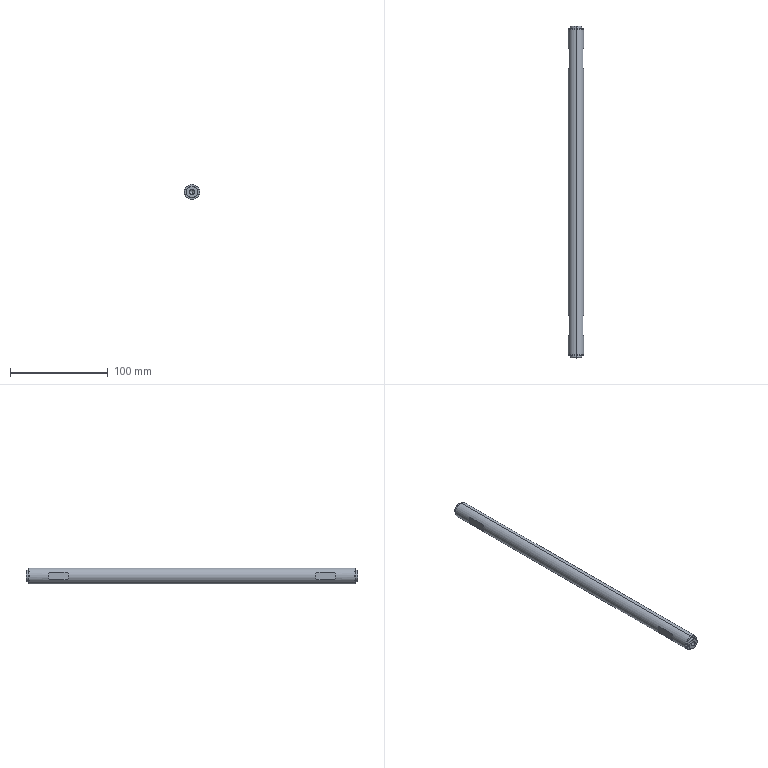Part | SolidWorks | features Chamfer 3, ICE 3, HoleWzd 2, Extrusion 1, MirrorPattern 1 | 1 solid | 38 faces | box 16 x 339 x 16 mm | volume 66505 mm3 | plane 16 | cone 12 | cylinder 10 | commonest cylinder face diameters 5 x4 12 x4 16 x2
STEP:
#1=CARTESIAN_POINT('',(0.,152.5,-2.5));
#2=VERTEX_POINT('',#1);
#3=CARTESIAN_POINT('',(0.,152.5,2.5));
#4=VERTEX_POINT('',#3);
#5=CARTESIAN_POINT('',(0.,152.5,0.));
#6=DIRECTION('',(0.,1.,0.));
#7=DIRECTION('',(0.,0.,1.));
#8=AXIS2_PLACEMENT_3D('',#5,#6,#7);
#9=CIRCLE('',#8,2.5);
#10=EDGE_CURVE('',#2,#4,#9,.T.);
#11=ORIENTED_EDGE('',*,*,#10,.F.);
#12=CARTESIAN_POINT('',(0.,169.5,-2.5));
#13=VERTEX_POINT('',#12);
#14=CARTESIAN_POINT('',(0.,169.5,-2.5));
#15=DIRECTION('',(0.,1.,0.));
#16=VECTOR('',#15,1000.);
#17=LINE('',#14,#16);
#18=EDGE_CURVE('',#2,#13,#17,.T.);
#19=ORIENTED_EDGE('',*,*,#18,.T.);
#20=CARTESIAN_POINT('',(0.,169.5,2.5));
#21=VERTEX_POINT('',#20);
#22=CARTESIAN_POINT('',(0.,169.5,0.));
#23=DIRECTION('',(0.,1.,0.));
#24=DIRECTION('',(0.,0.,1.));
#25=AXIS2_PLACEMENT_3D('',#22,#23,#24);
#26=CIRCLE('',#25,2.5);
#27=EDGE_CURVE('',#13,#21,#26,.T.);
#28=ORIENTED_EDGE('',*,*,#27,.T.);
#29=CARTESIAN_POINT('',(0.,169.5,2.5));
#30=DIRECTION('',(0.,1.,0.));
#31=VECTOR('',#30,1000.);
#32=LINE('',#29,#31);
#33=EDGE_CURVE('',#4,#21,#32,.T.);
#34=ORIENTED_EDGE('',*,*,#33,.F.);
#35=EDGE_LOOP('',(#11,#19,#28,#34));
#36=FACE_OUTER_BOUND('',#35,.T.);
#37=CARTESIAN_POINT('',(0.,169.5,0.));
#38=DIRECTION('',(0.,1.,0.));
#39=DIRECTION('',(0.,0.,1.));
#40=AXIS2_PLACEMENT_3D('',#37,#38,#39);
#41=CYLINDRICAL_SURFACE('',#40,2.5);
#42=ADVANCED_FACE('',(#36),#41,.F.);
#43=CARTESIAN_POINT('',(0.,150.998,0.));
#44=VERTEX_POINT('',#43);
#45=CARTESIAN_POINT('',(0.,152.5,2.5));
#46=DIRECTION('',(0.,0.515,0.8572));
#47=VECTOR('',#46,1000.);
#48=LINE('',#45,#47);
#49=EDGE_CURVE('',#44,#4,#48,.T.);
#50=ORIENTED_EDGE('',*,*,#49,.F.);
#51=CARTESIAN_POINT('',(0.,152.5,-2.5));
#52=DIRECTION('',(0.,0.515,-0.8572));
#53=VECTOR('',#52,1000.);
#54=LINE('',#51,#53);
#55=EDGE_CURVE('',#44,#2,#54,.T.);
#56=ORIENTED_EDGE('',*,*,#55,.T.);
#57=ORIENTED_EDGE('',*,*,#10,.T.);
#58=EDGE_LOOP('',(#50,#56,#57));
#59=FACE_OUTER_BOUND('',#58,.T.);
#60=CARTESIAN_POINT('',(0.,152.5,0.));
#61=DIRECTION('',(0.,1.,0.));
#62=DIRECTION('',(0.,0.,1.));
#63=AXIS2_PLACEMENT_3D('',#60,#61,#62);
#64=CONICAL_SURFACE('',#63,2.5,1.03);
#65=ADVANCED_FACE('',(#59),#64,.F.);
#66=CARTESIAN_POINT('',(0.,169.5,5.5));
#67=VERTEX_POINT('',#66);
#68=CARTESIAN_POINT('',(0.,169.5,-5.5));
#69=VERTEX_POINT('',#68);
#70=CARTESIAN_POINT('',(0.,169.5,0.));
#71=DIRECTION('',(0.,1.,0.));
#72=DIRECTION('',(0.,0.,1.));
#73=AXIS2_PLACEMENT_3D('',#70,#71,#72);
#74=CIRCLE('',#73,5.5);
#75=EDGE_CURVE('',#67,#69,#74,.T.);
#76=ORIENTED_EDGE('',*,*,#75,.F.);
#77=CARTESIAN_POINT('',(0.,169.,6.));
#78=VERTEX_POINT('',#77);
#79=CARTESIAN_POINT('',(0.,169.5,5.5));
#80=DIRECTION('',(0.,-0.7071,0.7071));
#81=VECTOR('',#80,1000.);
#82=LINE('',#79,#81);
#83=EDGE_CURVE('',#67,#78,#82,.T.);
#84=ORIENTED_EDGE('',*,*,#83,.T.);
#85=CARTESIAN_POINT('',(0.,169.,-6.));
#86=VERTEX_POINT('',#85);
#87=CARTESIAN_POINT('',(0.,169.,0.));
#88=DIRECTION('',(0.,-1.,0.));
#89=DIRECTION('',(0.,0.,1.));
#90=AXIS2_PLACEMENT_3D('',#87,#88,#89);
#91=CIRCLE('',#90,6.);
#92=EDGE_CURVE('',#86,#78,#91,.T.);
#93=ORIENTED_EDGE('',*,*,#92,.F.);
#94=CARTESIAN_POINT('',(0.,169.5,-5.5));
#95=DIRECTION('',(0.,-0.7071,-0.7071));
#96=VECTOR('',#95,1000.);
#97=LINE('',#94,#96);
#98=EDGE_CURVE('',#69,#86,#97,.T.);
#99=ORIENTED_EDGE('',*,*,#98,.F.);
#100=EDGE_LOOP('',(#76,#84,#93,#99));
#101=FACE_OUTER_BOUND('',#100,.T.);
#102=CARTESIAN_POINT('',(0.,169.5,0.));
#103=DIRECTION('',(0.,-1.,0.));
#104=DIRECTION('',(0.,0.,-1.));
#105=AXIS2_PLACEMENT_3D('',#102,#103,#104);
#106=CONICAL_SURFACE('',#105,5.5,0.7854);
#107=ADVANCED_FACE('',(#101),#106,.T.);
#108=ORIENTED_EDGE('',*,*,#92,.T.);
#109=CARTESIAN_POINT('',(0.,166.5,6.));
#110=VERTEX_POINT('',#109);
#111=CARTESIAN_POINT('',(0.,169.5,6.));
#112=DIRECTION('',(0.,-1.,0.));
#113=VECTOR('',#112,1000.);
#114=LINE('',#111,#113);
#115=EDGE_CURVE('',#78,#110,#114,.T.);
#116=ORIENTED_EDGE('',*,*,#115,.T.);
#117=CARTESIAN_POINT('',(0.,166.5,-6.));
#118=VERTEX_POINT('',#117);
#119=CARTESIAN_POINT('',(0.,166.5,0.));
#120=DIRECTION('',(0.,1.,0.));
#121=DIRECTION('',(0.,0.,1.));
#122=AXIS2_PLACEMENT_3D('',#119,#120,#121);
#123=CIRCLE('',#122,6.);
#124=EDGE_CURVE('',#110,#118,#123,.T.);
#125=ORIENTED_EDGE('',*,*,#124,.T.);
#126=CARTESIAN_POINT('',(0.,169.5,-6.));
#127=DIRECTION('',(0.,-1.,0.));
#128=VECTOR('',#127,1000.);
#129=LINE('',#126,#128);
#130=EDGE_CURVE('',#86,#118,#129,.T.);
#131=ORIENTED_EDGE('',*,*,#130,.F.);
#132=EDGE_LOOP('',(#108,#116,#125,#131));
#133=FACE_OUTER_BOUND('',#132,.T.);
#134=CARTESIAN_POINT('',(0.,169.5,0.));
#135=DIRECTION('',(0.,-1.,0.));
#136=DIRECTION('',(0.,0.,-1.));
#137=AXIS2_PLACEMENT_3D('',#134,#135,#136);
#138=CYLINDRICAL_SURFACE('',#137,6.);
#139=ADVANCED_FACE('',(#133),#138,.T.);
#140=CARTESIAN_POINT('',(0.,166.5,7.5));
#141=VERTEX_POINT('',#140);
#142=CARTESIAN_POINT('',(0.,166.5,-7.5));
#143=VERTEX_POINT('',#142);
#144=CARTESIAN_POINT('',(0.,166.5,0.));
#145=DIRECTION('',(0.,1.,0.));
#146=DIRECTION('',(0.,0.,1.));
#147=AXIS2_PLACEMENT_3D('',#144,#145,#146);
#148=CIRCLE('',#147,7.5);
#149=EDGE_CURVE('',#141,#143,#148,.T.);
#150=ORIENTED_EDGE('',*,*,#149,.F.);
#151=CARTESIAN_POINT('',(0.,166.,8.));
#152=VERTEX_POINT('',#151);
#153=CARTESIAN_POINT('',(0.,166.5,7.5));
#154=DIRECTION('',(0.,-0.7071,0.7071));
#155=VECTOR('',#154,1000.);
#156=LINE('',#153,#155);
#157=EDGE_CURVE('',#141,#152,#156,.T.);
#158=ORIENTED_EDGE('',*,*,#157,.T.);
#159=CARTESIAN_POINT('',(0.,166.,-8.));
#160=VERTEX_POINT('',#159);
#161=CARTESIAN_POINT('',(0.,166.,0.));
#162=DIRECTION('',(0.,-1.,0.));
#163=DIRECTION('',(0.,0.,1.));
#164=AXIS2_PLACEMENT_3D('',#161,#162,#163);
#165=CIRCLE('',#164,8.);
#166=EDGE_CURVE('',#160,#152,#165,.T.);
#167=ORIENTED_EDGE('',*,*,#166,.F.);
#168=CARTESIAN_POINT('',(0.,166.5,-7.5));
#169=DIRECTION('',(0.,-0.7071,-0.7071));
#170=VECTOR('',#169,1000.);
#171=LINE('',#168,#170);
#172=EDGE_CURVE('',#143,#160,#171,.T.);
#173=ORIENTED_EDGE('',*,*,#172,.F.);
#174=EDGE_LOOP('',(#150,#158,#167,#173));
#175=FACE_OUTER_BOUND('',#174,.T.);
#176=CARTESIAN_POINT('',(0.,166.5,0.));
#177=DIRECTION('',(0.,-1.,0.));
#178=DIRECTION('',(0.,0.,-1.));
#179=AXIS2_PLACEMENT_3D('',#176,#177,#178);
#180=CONICAL_SURFACE('',#179,7.5,0.7854);
#181=ADVANCED_FACE('',(#175),#180,.T.);
#182=CARTESIAN_POINT('',(0.,-152.5,2.5));
#183=VERTEX_POINT('',#182);
#184=CARTESIAN_POINT('',(0.,-152.5,-2.5));
#185=VERTEX_POINT('',#184);
#186=CARTESIAN_POINT('',(0.,-152.5,0.));
#187=DIRECTION('',(0.,-1.,0.));
#188=DIRECTION('',(0.,0.,-1.));
#189=AXIS2_PLACEMENT_3D('',#186,#187,#188);
#190=CIRCLE('',#189,2.5);
#191=EDGE_CURVE('',#183,#185,#190,.T.);
#192=ORIENTED_EDGE('',*,*,#191,.F.);
#193=CARTESIAN_POINT('',(0.,-169.5,2.5));
#194=VERTEX_POINT('',#193);
#195=CARTESIAN_POINT('',(0.,-169.5,2.5));
#196=DIRECTION('',(0.,-1.,0.));
#197=VECTOR('',#196,1000.);
#198=LINE('',#195,#197);
#199=EDGE_CURVE('',#183,#194,#198,.T.);
#200=ORIENTED_EDGE('',*,*,#199,.T.);
#201=CARTESIAN_POINT('',(0.,-169.5,-2.5));
#202=VERTEX_POINT('',#201);
#203=CARTESIAN_POINT('',(0.,-169.5,0.));
#204=DIRECTION('',(0.,-1.,0.));
#205=DIRECTION('',(0.,0.,-1.));
#206=AXIS2_PLACEMENT_3D('',#203,#204,#205);
#207=CIRCLE('',#206,2.5);
#208=EDGE_CURVE('',#194,#202,#207,.T.);
#209=ORIENTED_EDGE('',*,*,#208,.T.);
#210=CARTESIAN_POINT('',(0.,-169.5,-2.5));
#211=DIRECTION('',(0.,-1.,0.));
#212=VECTOR('',#211,1000.);
#213=LINE('',#210,#212);
#214=EDGE_CURVE('',#185,#202,#213,.T.);
#215=ORIENTED_EDGE('',*,*,#214,.F.);
#216=EDGE_LOOP('',(#192,#200,#209,#215));
#217=FACE_OUTER_BOUND('',#216,.T.);
#218=CARTESIAN_POINT('',(0.,-169.5,0.));
#219=DIRECTION('',(0.,-1.,0.));
#220=DIRECTION('',(0.,0.,-1.));
#221=AXIS2_PLACEMENT_3D('',#218,#219,#220);
#222=CYLINDRICAL_SURFACE('',#221,2.5);
#223=ADVANCED_FACE('',(#217),#222,.F.);
#224=CARTESIAN_POINT('',(0.,-150.998,0.));
#225=VERTEX_POINT('',#224);
#226=CARTESIAN_POINT('',(0.,-152.5,-2.5));
#227=DIRECTION('',(0.,-0.515,-0.8572));
#228=VECTOR('',#227,1000.);
#229=LINE('',#226,#228);
#230=EDGE_CURVE('',#225,#185,#229,.T.);
#231=ORIENTED_EDGE('',*,*,#230,.F.);
#232=CARTESIAN_POINT('',(0.,-152.5,2.5));
#233=DIRECTION('',(0.,-0.515,0.8572));
#234=VECTOR('',#233,1000.);
#235=LINE('',#232,#234);
#236=EDGE_CURVE('',#225,#183,#235,.T.);
#237=ORIENTED_EDGE('',*,*,#236,.T.);
#238=ORIENTED_EDGE('',*,*,#191,.T.);
#239=EDGE_LOOP('',(#231,#237,#238));
#240=FACE_OUTER_BOUND('',#239,.T.);
#241=CARTESIAN_POINT('',(0.,-152.5,0.));
#242=DIRECTION('',(0.,-1.,0.));
#243=DIRECTION('',(0.,0.,-1.));
#244=AXIS2_PLACEMENT_3D('',#241,#242,#243);
#245=CONICAL_SURFACE('',#244,2.5,1.03);
#246=ADVANCED_FACE('',(#240),#245,.F.);
#247=CARTESIAN_POINT('',(0.,-166.5,-7.5));
#248=VERTEX_POINT('',#247);
#249=CARTESIAN_POINT('',(0.,-166.5,7.5));
#250=VERTEX_POINT('',#249);
#251=CARTESIAN_POINT('',(0.,-166.5,0.));
#252=DIRECTION('',(0.,-1.,0.));
#253=DIRECTION('',(0.,0.,1.));
#254=AXIS2_PLACEMENT_3D('',#251,#252,#253);
#255=CIRCLE('',#254,7.5);
#256=EDGE_CURVE('',#248,#250,#255,.T.);
#257=ORIENTED_EDGE('',*,*,#256,.F.);
#258=CARTESIAN_POINT('',(0.,-166.,-8.));
#259=VERTEX_POINT('',#258);
#260=CARTESIAN_POINT('',(0.,-166.,-8.));
#261=DIRECTION('',(0.,0.7071,-0.7071));
#262=VECTOR('',#261,1000.);
#263=LINE('',#260,#262);
#264=EDGE_CURVE('',#248,#259,#263,.T.);
#265=ORIENTED_EDGE('',*,*,#264,.T.);
#266=CARTESIAN_POINT('',(0.,-166.,8.));
#267=VERTEX_POINT('',#266);
#268=CARTESIAN_POINT('',(0.,-166.,0.));
#269=DIRECTION('',(0.,1.,0.));
#270=DIRECTION('',(0.,0.,1.));
#271=AXIS2_PLACEMENT_3D('',#268,#269,#270);
#272=CIRCLE('',#271,8.);
#273=EDGE_CURVE('',#267,#259,#272,.T.);
#274=ORIENTED_EDGE('',*,*,#273,.F.);
#275=CARTESIAN_POINT('',(0.,-166.,8.));
#276=DIRECTION('',(0.,0.7071,0.7071));
#277=VECTOR('',#276,1000.);
#278=LINE('',#275,#277);
#279=EDGE_CURVE('',#250,#267,#278,.T.);
#280=ORIENTED_EDGE('',*,*,#279,.F.);
#281=EDGE_LOOP('',(#257,#265,#274,#280));
#282=FACE_OUTER_BOUND('',#281,.T.);
#283=CARTESIAN_POINT('',(0.,-166.,0.));
#284=DIRECTION('',(0.,1.,0.));
#285=DIRECTION('',(0.,0.,1.));
#286=AXIS2_PLACEMENT_3D('',#283,#284,#285);
#287=CONICAL_SURFACE('',#286,8.,0.7854);
#288=ADVANCED_FACE('',(#282),#287,.T.);
#289=CARTESIAN_POINT('',(0.,-169.5,-5.5));
#290=VERTEX_POINT('',#289);
#291=CARTESIAN_POINT('',(0.,-169.5,5.5));
#292=VERTEX_POINT('',#291);
#293=CARTESIAN_POINT('',(0.,-169.5,0.));
#294=DIRECTION('',(0.,-1.,0.));
#295=DIRECTION('',(0.,0.,-1.));
#296=AXIS2_PLACEMENT_3D('',#293,#294,#295);
#297=CIRCLE('',#296,5.5);
#298=EDGE_CURVE('',#290,#292,#297,.T.);
#299=ORIENTED_EDGE('',*,*,#298,.F.);
#300=CARTESIAN_POINT('',(0.,-169.,-6.));
#301=VERTEX_POINT('',#300);
#302=CARTESIAN_POINT('',(0.,-169.5,-5.5));
#303=DIRECTION('',(0.,0.7071,-0.7071));
#304=VECTOR('',#303,1000.);
#305=LINE('',#302,#304);
#306=EDGE_CURVE('',#290,#301,#305,.T.);
#307=ORIENTED_EDGE('',*,*,#306,.T.);
#308=CARTESIAN_POINT('',(0.,-169.,6.));
#309=VERTEX_POINT('',#308);
#310=CARTESIAN_POINT('',(0.,-169.,0.));
#311=DIRECTION('',(0.,1.,0.));
#312=DIRECTION('',(0.,0.,-1.));
#313=AXIS2_PLACEMENT_3D('',#310,#311,#312);
#314=CIRCLE('',#313,6.);
#315=EDGE_CURVE('',#309,#301,#314,.T.);
#316=ORIENTED_EDGE('',*,*,#315,.F.);
#317=CARTESIAN_POINT('',(0.,-169.5,5.5));
#318=DIRECTION('',(0.,0.7071,0.7071));
#319=VECTOR('',#318,1000.);
#320=LINE('',#317,#319);
#321=EDGE_CURVE('',#292,#309,#320,.T.);
#322=ORIENTED_EDGE('',*,*,#321,.F.);
#323=EDGE_LOOP('',(#299,#307,#316,#322));
#324=FACE_OUTER_BOUND('',#323,.T.);
#325=CARTESIAN_POINT('',(0.,-169.5,0.));
#326=DIRECTION('',(0.,1.,0.));
#327=DIRECTION('',(0.,0.,1.));
#328=AXIS2_PLACEMENT_3D('',#325,#326,#327);
#329=CONICAL_SURFACE('',#328,5.5,0.7854);
#330=ADVANCED_FACE('',(#324),#329,.T.);
#331=ORIENTED_EDGE('',*,*,#315,.T.);
#332=CARTESIAN_POINT('',(0.,-166.5,-6.));
#333=VERTEX_POINT('',#332);
#334=CARTESIAN_POINT('',(0.,-169.5,-6.));
#335=DIRECTION('',(0.,1.,0.));
#336=VECTOR('',#335,1000.);
#337=LINE('',#334,#336);
#338=EDGE_CURVE('',#301,#333,#337,.T.);
#339=ORIENTED_EDGE('',*,*,#338,.T.);
#340=CARTESIAN_POINT('',(0.,-166.5,6.));
#341=VERTEX_POINT('',#340);
#342=CARTESIAN_POINT('',(0.,-166.5,0.));
#343=DIRECTION('',(0.,-1.,0.));
#344=DIRECTION('',(0.,0.,1.));
#345=AXIS2_PLACEMENT_3D('',#342,#343,#344);
#346=CIRCLE('',#345,6.);
#347=EDGE_CURVE('',#333,#341,#346,.T.);
#348=ORIENTED_EDGE('',*,*,#347,.T.);
#349=CARTESIAN_POINT('',(0.,-169.5,6.));
#350=DIRECTION('',(0.,1.,0.));
#351=VECTOR('',#350,1000.);
#352=LINE('',#349,#351);
#353=EDGE_CURVE('',#309,#341,#352,.T.);
#354=ORIENTED_EDGE('',*,*,#353,.F.);
#355=EDGE_LOOP('',(#331,#339,#348,#354));
#356=FACE_OUTER_BOUND('',#355,.T.);
#357=CARTESIAN_POINT('',(0.,-169.5,0.));
#358=DIRECTION('',(0.,1.,0.));
#359=DIRECTION('',(0.,0.,1.));
#360=AXIS2_PLACEMENT_3D('',#357,#358,#359);
#361=CYLINDRICAL_SURFACE('',#360,6.);
#362=ADVANCED_FACE('',(#356),#361,.T.);
#363=CARTESIAN_POINT('',(7.,126.5,-3.873));
#364=VERTEX_POINT('',#363);
#365=CARTESIAN_POINT('',(7.,126.5,3.873));
#366=VERTEX_POINT('',#365);
#367=CARTESIAN_POINT('',(0.,126.5,0.));
#368=DIRECTION('',(0.,-1.,0.));
#369=DIRECTION('',(0.,0.,-1.));
#370=AXIS2_PLACEMENT_3D('',#367,#368,#369);
#371=CIRCLE('',#370,8.);
#372=EDGE_CURVE('',#364,#366,#371,.T.);
#373=ORIENTED_EDGE('',*,*,#372,.T.);
#374=CARTESIAN_POINT('',(7.,146.5,3.873));
#375=VERTEX_POINT('',#374);
#376=CARTESIAN_POINT('',(7.,126.5,3.873));
#377=DIRECTION('',(0.,1.,0.));
#378=VECTOR('',#377,1000.);
#379=LINE('',#376,#378);
#380=EDGE_CURVE('',#366,#375,#379,.T.);
#381=ORIENTED_EDGE('',*,*,#380,.T.);
#382=CARTESIAN_POINT('',(7.,146.5,-3.873));
#383=VERTEX_POINT('',#382);
#384=CARTESIAN_POINT('',(0.,146.5,0.));
#385=DIRECTION('',(0.,-1.,0.));
#386=DIRECTION('',(0.,0.,-1.));
#387=AXIS2_PLACEMENT_3D('',#384,#385,#386);
#388=CIRCLE('',#387,8.);
#389=EDGE_CURVE('',#383,#375,#388,.T.);
#390=ORIENTED_EDGE('',*,*,#389,.F.);
#391=CARTESIAN_POINT('',(7.,126.5,-3.873));
#392=DIRECTION('',(0.,1.,0.));
#393=VECTOR('',#392,1000.);
#394=LINE('',#391,#393);
#395=EDGE_CURVE('',#364,#383,#394,.T.);
#396=ORIENTED_EDGE('',*,*,#395,.F.);
#397=EDGE_LOOP('',(#373,#381,#390,#396));
#398=FACE_BOUND('',#397,.T.);
#399=CARTESIAN_POINT('',(7.,-126.5,-3.873));
#400=VERTEX_POINT('',#399);
#401=CARTESIAN_POINT('',(7.,-126.5,3.873));
#402=VERTEX_POINT('',#401);
#403=CARTESIAN_POINT('',(0.,-126.5,0.));
#404=DIRECTION('',(0.,-1.,0.));
#405=DIRECTION('',(0.,0.,-1.));
#406=AXIS2_PLACEMENT_3D('',#403,#404,#405);
#407=CIRCLE('',#406,8.);
#408=EDGE_CURVE('',#400,#402,#407,.T.);
#409=ORIENTED_EDGE('',*,*,#408,.F.);
#410=CARTESIAN_POINT('',(7.,-146.5,-3.873));
#411=VERTEX_POINT('',#410);
#412=CARTESIAN_POINT('',(7.,-126.5,-3.873));
#413=DIRECTION('',(0.,-1.,0.));
#414=VECTOR('',#413,1000.);
#415=LINE('',#412,#414);
#416=EDGE_CURVE('',#400,#411,#415,.T.);
#417=ORIENTED_EDGE('',*,*,#416,.T.);
#418=CARTESIAN_POINT('',(7.,-146.5,3.873));
#419=VERTEX_POINT('',#418);
#420=CARTESIAN_POINT('',(0.,-146.5,0.));
#421=DIRECTION('',(0.,-1.,0.));
#422=DIRECTION('',(0.,0.,-1.));
#423=AXIS2_PLACEMENT_3D('',#420,#421,#422);
#424=CIRCLE('',#423,8.);
#425=EDGE_CURVE('',#411,#419,#424,.T.);
#426=ORIENTED_EDGE('',*,*,#425,.T.);
#427=CARTESIAN_POINT('',(7.,-126.5,3.873));
#428=DIRECTION('',(0.,-1.,0.));
#429=VECTOR('',#428,1000.);
#430=LINE('',#427,#429);
#431=EDGE_CURVE('',#402,#419,#430,.T.);
#432=ORIENTED_EDGE('',*,*,#431,.F.);
#433=EDGE_LOOP('',(#409,#417,#426,#432));
#434=FACE_BOUND('',#433,.T.);
#435=ORIENTED_EDGE('',*,*,#166,.T.);
#436=CARTESIAN_POINT('',(0.,166.5,8.));
#437=DIRECTION('',(0.,-1.,0.));
#438=VECTOR('',#437,1000.);
#439=LINE('',#436,#438);
#440=EDGE_CURVE('',#152,#267,#439,.T.);
#441=ORIENTED_EDGE('',*,*,#440,.T.);
#442=ORIENTED_EDGE('',*,*,#273,.T.);
#443=CARTESIAN_POINT('',(0.,166.5,-8.));
#444=DIRECTION('',(0.,-1.,0.));
#445=VECTOR('',#444,1000.);
#446=LINE('',#443,#445);
#447=EDGE_CURVE('',#160,#259,#446,.T.);
#448=ORIENTED_EDGE('',*,*,#447,.F.);
#449=EDGE_LOOP('',(#435,#441,#442,#448));
#450=FACE_OUTER_BOUND('',#449,.T.);
#451=CARTESIAN_POINT('',(0.,166.5,0.));
#452=DIRECTION('',(0.,-1.,0.));
#453=DIRECTION('',(0.,0.,-1.));
#454=AXIS2_PLACEMENT_3D('',#451,#452,#453);
#455=CYLINDRICAL_SURFACE('',#454,8.);
#456=ADVANCED_FACE('',(#398,#434,#450),#455,.T.);
#457=ORIENTED_EDGE('',*,*,#440,.F.);
#458=CARTESIAN_POINT('',(0.,166.,0.));
#459=DIRECTION('',(0.,-1.,0.));
#460=DIRECTION('',(0.,0.,1.));
#461=AXIS2_PLACEMENT_3D('',#458,#459,#460);
#462=CIRCLE('',#461,8.);
#463=EDGE_CURVE('',#152,#160,#462,.T.);
#464=ORIENTED_EDGE('',*,*,#463,.T.);
#465=ORIENTED_EDGE('',*,*,#447,.T.);
#466=CARTESIAN_POINT('',(0.,-166.,0.));
#467=DIRECTION('',(0.,1.,0.));
#468=DIRECTION('',(0.,0.,1.));
#469=AXIS2_PLACEMENT_3D('',#466,#467,#468);
#470=CIRCLE('',#469,8.);
#471=EDGE_CURVE('',#259,#267,#470,.T.);
#472=ORIENTED_EDGE('',*,*,#471,.T.);
#473=EDGE_LOOP('',(#457,#464,#465,#472));
#474=FACE_OUTER_BOUND('',#473,.T.);
#475=CARTESIAN_POINT('',(-7.,126.5,3.873));
#476=VERTEX_POINT('',#475);
#477=CARTESIAN_POINT('',(-7.,126.5,-3.873));
#478=VERTEX_POINT('',#477);
#479=CARTESIAN_POINT('',(0.,126.5,0.));
#480=DIRECTION('',(0.,-1.,0.));
#481=DIRECTION('',(0.,0.,-1.));
#482=AXIS2_PLACEMENT_3D('',#479,#480,#481);
#483=CIRCLE('',#482,8.);
#484=EDGE_CURVE('',#476,#478,#483,.T.);
#485=ORIENTED_EDGE('',*,*,#484,.T.);
#486=CARTESIAN_POINT('',(-7.,146.5,-3.873));
#487=VERTEX_POINT('',#486);
#488=CARTESIAN_POINT('',(-7.,126.5,-3.873));
#489=DIRECTION('',(0.,1.,0.));
#490=VECTOR('',#489,1000.);
#491=LINE('',#488,#490);
#492=EDGE_CURVE('',#478,#487,#491,.T.);
#493=ORIENTED_EDGE('',*,*,#492,.T.);
#494=CARTESIAN_POINT('',(-7.,146.5,3.873));
#495=VERTEX_POINT('',#494);
#496=CARTESIAN_POINT('',(0.,146.5,0.));
#497=DIRECTION('',(0.,-1.,0.));
#498=DIRECTION('',(0.,0.,-1.));
#499=AXIS2_PLACEMENT_3D('',#496,#497,#498);
#500=CIRCLE('',#499,8.);
#501=EDGE_CURVE('',#495,#487,#500,.T.);
#502=ORIENTED_EDGE('',*,*,#501,.F.);
#503=CARTESIAN_POINT('',(-7.,126.5,3.873));
#504=DIRECTION('',(0.,1.,0.));
#505=VECTOR('',#504,1000.);
#506=LINE('',#503,#505);
#507=EDGE_CURVE('',#476,#495,#506,.T.);
#508=ORIENTED_EDGE('',*,*,#507,.F.);
#509=EDGE_LOOP('',(#485,#493,#502,#508));
#510=FACE_BOUND('',#509,.T.);
#511=CARTESIAN_POINT('',(-7.,-126.5,3.873));
#512=VERTEX_POINT('',#511);
#513=CARTESIAN_POINT('',(-7.,-126.5,-3.873));
#514=VERTEX_POINT('',#513);
#515=CARTESIAN_POINT('',(0.,-126.5,0.));
#516=DIRECTION('',(0.,-1.,0.));
#517=DIRECTION('',(0.,0.,-1.));
#518=AXIS2_PLACEMENT_3D('',#515,#516,#517);
#519=CIRCLE('',#518,8.);
#520=EDGE_CURVE('',#512,#514,#519,.T.);
#521=ORIENTED_EDGE('',*,*,#520,.F.);
#522=CARTESIAN_POINT('',(-7.,-146.5,3.873));
#523=VERTEX_POINT('',#522);
#524=CARTESIAN_POINT('',(-7.,-126.5,3.873));
#525=DIRECTION('',(0.,-1.,0.));
#526=VECTOR('',#525,1000.);
#527=LINE('',#524,#526);
#528=EDGE_CURVE('',#512,#523,#527,.T.);
#529=ORIENTED_EDGE('',*,*,#528,.T.);
#530=CARTESIAN_POINT('',(-7.,-146.5,-3.873));
#531=VERTEX_POINT('',#530);
#532=CARTESIAN_POINT('',(0.,-146.5,0.));
#533=DIRECTION('',(0.,-1.,0.));
#534=DIRECTION('',(0.,0.,-1.));
#535=AXIS2_PLACEMENT_3D('',#532,#533,#534);
#536=CIRCLE('',#535,8.);
#537=EDGE_CURVE('',#523,#531,#536,.T.);
#538=ORIENTED_EDGE('',*,*,#537,.T.);
#539=CARTESIAN_POINT('',(-7.,-126.5,-3.873));
#540=DIRECTION('',(0.,-1.,0.));
#541=VECTOR('',#540,1000.);
#542=LINE('',#539,#541);
#543=EDGE_CURVE('',#514,#531,#542,.T.);
#544=ORIENTED_EDGE('',*,*,#543,.F.);
#545=EDGE_LOOP('',(#521,#529,#538,#544));
#546=FACE_BOUND('',#545,.T.);
#547=CARTESIAN_POINT('',(0.,166.5,0.));
#548=DIRECTION('',(0.,-1.,0.));
#549=DIRECTION('',(0.,0.,-1.));
#550=AXIS2_PLACEMENT_3D('',#547,#548,#549);
#551=CYLINDRICAL_SURFACE('',#550,8.);
#552=ADVANCED_FACE('',(#474,#510,#546),#551,.T.);
#553=CARTESIAN_POINT('',(0.,166.5,0.));
#554=DIRECTION('',(0.,1.,0.));
#555=DIRECTION('',(0.,0.,1.));
#556=AXIS2_PLACEMENT_3D('',#553,#554,#555);
#557=CIRCLE('',#556,7.5);
#558=EDGE_CURVE('',#143,#141,#557,.T.);
#559=ORIENTED_EDGE('',*,*,#558,.T.);
#560=ORIENTED_EDGE('',*,*,#149,.T.);
#561=EDGE_LOOP('',(#559,#560));
#562=FACE_OUTER_BOUND('',#561,.T.);
#563=CARTESIAN_POINT('',(0.,166.5,0.));
#564=DIRECTION('',(0.,1.,0.));
#565=DIRECTION('',(0.,0.,1.));
#566=AXIS2_PLACEMENT_3D('',#563,#564,#565);
#567=CIRCLE('',#566,6.);
#568=EDGE_CURVE('',#118,#110,#567,.T.);
#569=ORIENTED_EDGE('',*,*,#568,.F.);
#570=ORIENTED_EDGE('',*,*,#124,.F.);
#571=EDGE_LOOP('',(#569,#570));
#572=FACE_BOUND('',#571,.T.);
#573=CARTESIAN_POINT('',(0.,166.5,0.));
#574=DIRECTION('',(0.,1.,0.));
#575=DIRECTION('',(0.,0.,1.));
#576=AXIS2_PLACEMENT_3D('',#573,#574,#575);
#577=PLANE('',#576);
#578=ADVANCED_FACE('',(#562,#572),#577,.T.);
#579=CARTESIAN_POINT('',(0.,-166.5,0.));
#580=DIRECTION('',(0.,-1.,0.));
#581=DIRECTION('',(0.,0.,1.));
#582=AXIS2_PLACEMENT_3D('',#579,#580,#581);
#583=CIRCLE('',#582,7.5);
#584=EDGE_CURVE('',#250,#248,#583,.T.);
#585=ORIENTED_EDGE('',*,*,#584,.T.);
#586=ORIENTED_EDGE('',*,*,#256,.T.);
#587=EDGE_LOOP('',(#585,#586));
#588=FACE_OUTER_BOUND('',#587,.T.);
#589=CARTESIAN_POINT('',(0.,-166.5,0.));
#590=DIRECTION('',(0.,-1.,0.));
#591=DIRECTION('',(0.,0.,1.));
#592=AXIS2_PLACEMENT_3D('',#589,#590,#591);
#593=CIRCLE('',#592,6.);
#594=EDGE_CURVE('',#341,#333,#593,.T.);
#595=ORIENTED_EDGE('',*,*,#594,.F.);
#596=ORIENTED_EDGE('',*,*,#347,.F.);
#597=EDGE_LOOP('',(#595,#596));
#598=FACE_BOUND('',#597,.T.);
#599=CARTESIAN_POINT('',(0.,-166.5,0.));
#600=DIRECTION('',(0.,1.,0.));
#601=DIRECTION('',(0.,0.,1.));
#602=AXIS2_PLACEMENT_3D('',#599,#600,#601);
#603=PLANE('',#602);
#604=ADVANCED_FACE('',(#588,#598),#603,.F.);
#605=ORIENTED_EDGE('',*,*,#338,.F.);
#606=CARTESIAN_POINT('',(0.,-169.,0.));
#607=DIRECTION('',(0.,1.,0.));
#608=DIRECTION('',(0.,0.,-1.));
#609=AXIS2_PLACEMENT_3D('',#606,#607,#608);
#610=CIRCLE('',#609,6.);
#611=EDGE_CURVE('',#301,#309,#610,.T.);
#612=ORIENTED_EDGE('',*,*,#611,.T.);
#613=ORIENTED_EDGE('',*,*,#353,.T.);
#614=ORIENTED_EDGE('',*,*,#594,.T.);
#615=EDGE_LOOP('',(#605,#612,#613,#614));
#616=FACE_OUTER_BOUND('',#615,.T.);
#617=CARTESIAN_POINT('',(0.,-169.5,0.));
#618=DIRECTION('',(0.,1.,0.));
#619=DIRECTION('',(0.,0.,1.));
#620=AXIS2_PLACEMENT_3D('',#617,#618,#619);
#621=CYLINDRICAL_SURFACE('',#620,6.);
#622=ADVANCED_FACE('',(#616),#621,.T.);
#623=CARTESIAN_POINT('',(0.,-169.5,0.));
#624=DIRECTION('',(0.,-1.,0.));
#625=DIRECTION('',(0.,0.,-1.));
#626=AXIS2_PLACEMENT_3D('',#623,#624,#625);
#627=CIRCLE('',#626,2.5);
#628=EDGE_CURVE('',#202,#194,#627,.T.);
#629=ORIENTED_EDGE('',*,*,#628,.F.);
#630=ORIENTED_EDGE('',*,*,#208,.F.);
#631=EDGE_LOOP('',(#629,#630));
#632=FACE_BOUND('',#631,.T.);
#633=CARTESIAN_POINT('',(0.,-169.5,0.));
#634=DIRECTION('',(0.,-1.,0.));
#635=DIRECTION('',(0.,0.,-1.));
#636=AXIS2_PLACEMENT_3D('',#633,#634,#635);
#637=CIRCLE('',#636,5.5);
#638=EDGE_CURVE('',#292,#290,#637,.T.);
#639=ORIENTED_EDGE('',*,*,#638,.T.);
#640=ORIENTED_EDGE('',*,*,#298,.T.);
#641=EDGE_LOOP('',(#639,#640));
#642=FACE_OUTER_BOUND('',#641,.T.);
#643=CARTESIAN_POINT('',(0.,-169.5,0.));
#644=DIRECTION('',(0.,-1.,0.));
#645=DIRECTION('',(0.,0.,-1.));
#646=AXIS2_PLACEMENT_3D('',#643,#644,#645);
#647=PLANE('',#646);
#648=ADVANCED_FACE('',(#632,#642),#647,.T.);
#649=ORIENTED_EDGE('',*,*,#306,.F.);
#650=ORIENTED_EDGE('',*,*,#638,.F.);
#651=ORIENTED_EDGE('',*,*,#321,.T.);
#652=ORIENTED_EDGE('',*,*,#611,.F.);
#653=EDGE_LOOP('',(#649,#650,#651,#652));
#654=FACE_OUTER_BOUND('',#653,.T.);
#655=CARTESIAN_POINT('',(0.,-169.5,0.));
#656=DIRECTION('',(0.,1.,0.));
#657=DIRECTION('',(0.,0.,1.));
#658=AXIS2_PLACEMENT_3D('',#655,#656,#657);
#659=CONICAL_SURFACE('',#658,5.5,0.7854);
#660=ADVANCED_FACE('',(#654),#659,.T.);
#661=ORIENTED_EDGE('',*,*,#264,.F.);
#662=ORIENTED_EDGE('',*,*,#584,.F.);
#663=ORIENTED_EDGE('',*,*,#279,.T.);
#664=ORIENTED_EDGE('',*,*,#471,.F.);
#665=EDGE_LOOP('',(#661,#662,#663,#664));
#666=FACE_OUTER_BOUND('',#665,.T.);
#667=CARTESIAN_POINT('',(0.,-166.,0.));
#668=DIRECTION('',(0.,1.,0.));
#669=DIRECTION('',(0.,0.,1.));
#670=AXIS2_PLACEMENT_3D('',#667,#668,#669);
#671=CONICAL_SURFACE('',#670,8.,0.7854);
#672=ADVANCED_FACE('',(#666),#671,.T.);
#673=CARTESIAN_POINT('',(-7.,-146.5,3.873));
#674=DIRECTION('',(0.,0.,1.));
#675=VECTOR('',#674,1000.);
#676=LINE('',#673,#675);
#677=EDGE_CURVE('',#531,#523,#676,.T.);
#678=ORIENTED_EDGE('',*,*,#677,.T.);
#679=ORIENTED_EDGE('',*,*,#528,.F.);
#680=CARTESIAN_POINT('',(-7.,-126.5,3.873));
#681=DIRECTION('',(0.,0.,1.));
#682=VECTOR('',#681,1000.);
#683=LINE('',#680,#682);
#684=EDGE_CURVE('',#514,#512,#683,.T.);
#685=ORIENTED_EDGE('',*,*,#684,.F.);
#686=ORIENTED_EDGE('',*,*,#543,.T.);
#687=EDGE_LOOP('',(#678,#679,#685,#686));
#688=FACE_OUTER_BOUND('',#687,.T.);
#689=CARTESIAN_POINT('',(-7.,-126.5,3.873));
#690=DIRECTION('',(1.,0.,0.));
#691=DIRECTION('',(0.,0.,-1.));
#692=AXIS2_PLACEMENT_3D('',#689,#690,#691);
#693=PLANE('',#692);
#694=ADVANCED_FACE('',(#688),#693,.F.);
#695=ORIENTED_EDGE('',*,*,#520,.T.);
#696=ORIENTED_EDGE('',*,*,#684,.T.);
#697=EDGE_LOOP('',(#695,#696));
#698=FACE_OUTER_BOUND('',#697,.T.);
#699=CARTESIAN_POINT('',(0.,-126.5,0.));
#700=DIRECTION('',(0.,-1.,0.));
#701=DIRECTION('',(0.,0.,-1.));
#702=AXIS2_PLACEMENT_3D('',#699,#700,#701);
#703=PLANE('',#702);
#704=ADVANCED_FACE('',(#698),#703,.T.);
#705=ORIENTED_EDGE('',*,*,#537,.F.);
#706=ORIENTED_EDGE('',*,*,#677,.F.);
#707=EDGE_LOOP('',(#705,#706));
#708=FACE_OUTER_BOUND('',#707,.T.);
#709=CARTESIAN_POINT('',(0.,-146.5,0.));
#710=DIRECTION('',(0.,-1.,0.));
#711=DIRECTION('',(0.,0.,-1.));
#712=AXIS2_PLACEMENT_3D('',#709,#710,#711);
#713=PLANE('',#712);
#714=ADVANCED_FACE('',(#708),#713,.F.);
#715=CARTESIAN_POINT('',(7.,-146.5,3.873));
#716=DIRECTION('',(0.,0.,-1.));
#717=VECTOR('',#716,1000.);
#718=LINE('',#715,#717);
#719=EDGE_CURVE('',#419,#411,#718,.T.);
#720=ORIENTED_EDGE('',*,*,#719,.T.);
#721=ORIENTED_EDGE('',*,*,#416,.F.);
#722=CARTESIAN_POINT('',(7.,-126.5,3.873));
#723=DIRECTION('',(0.,0.,-1.));
#724=VECTOR('',#723,1000.);
#725=LINE('',#722,#724);
#726=EDGE_CURVE('',#402,#400,#725,.T.);
#727=ORIENTED_EDGE('',*,*,#726,.F.);
#728=ORIENTED_EDGE('',*,*,#431,.T.);
#729=EDGE_LOOP('',(#720,#721,#727,#728));
#730=FACE_OUTER_BOUND('',#729,.T.);
#731=CARTESIAN_POINT('',(7.,-126.5,3.873));
#732=DIRECTION('',(-1.,0.,0.));
#733=DIRECTION('',(0.,0.,1.));
#734=AXIS2_PLACEMENT_3D('',#731,#732,#733);
#735=PLANE('',#734);
#736=ADVANCED_FACE('',(#730),#735,.F.);
#737=ORIENTED_EDGE('',*,*,#408,.T.);
#738=ORIENTED_EDGE('',*,*,#726,.T.);
#739=EDGE_LOOP('',(#737,#738));
#740=FACE_OUTER_BOUND('',#739,.T.);
#741=CARTESIAN_POINT('',(0.,-126.5,0.));
#742=DIRECTION('',(0.,-1.,0.));
#743=DIRECTION('',(0.,0.,-1.));
#744=AXIS2_PLACEMENT_3D('',#741,#742,#743);
#745=PLANE('',#744);
#746=ADVANCED_FACE('',(#740),#745,.T.);
#747=ORIENTED_EDGE('',*,*,#425,.F.);
#748=ORIENTED_EDGE('',*,*,#719,.F.);
#749=EDGE_LOOP('',(#747,#748));
#750=FACE_OUTER_BOUND('',#749,.T.);
#751=CARTESIAN_POINT('',(0.,-146.5,0.));
#752=DIRECTION('',(0.,-1.,0.));
#753=DIRECTION('',(0.,0.,-1.));
#754=AXIS2_PLACEMENT_3D('',#751,#752,#753);
#755=PLANE('',#754);
#756=ADVANCED_FACE('',(#750),#755,.F.);
#757=ORIENTED_EDGE('',*,*,#236,.F.);
#758=ORIENTED_EDGE('',*,*,#230,.T.);
#759=CARTESIAN_POINT('',(0.,-152.5,0.));
#760=DIRECTION('',(0.,-1.,0.));
#761=DIRECTION('',(0.,0.,-1.));
#762=AXIS2_PLACEMENT_3D('',#759,#760,#761);
#763=CIRCLE('',#762,2.5);
#764=EDGE_CURVE('',#185,#183,#763,.T.);
#765=ORIENTED_EDGE('',*,*,#764,.T.);
#766=EDGE_LOOP('',(#757,#758,#765));
#767=FACE_OUTER_BOUND('',#766,.T.);
#768=CARTESIAN_POINT('',(0.,-152.5,0.));
#769=DIRECTION('',(0.,-1.,0.));
#770=DIRECTION('',(0.,0.,-1.));
#771=AXIS2_PLACEMENT_3D('',#768,#769,#770);
#772=CONICAL_SURFACE('',#771,2.5,1.03);
#773=ADVANCED_FACE('',(#767),#772,.F.);
#774=ORIENTED_EDGE('',*,*,#199,.F.);
#775=ORIENTED_EDGE('',*,*,#764,.F.);
#776=ORIENTED_EDGE('',*,*,#214,.T.);
#777=ORIENTED_EDGE('',*,*,#628,.T.);
#778=EDGE_LOOP('',(#774,#775,#776,#777));
#779=FACE_OUTER_BOUND('',#778,.T.);
#780=CARTESIAN_POINT('',(0.,-169.5,0.));
#781=DIRECTION('',(0.,-1.,0.));
#782=DIRECTION('',(0.,0.,-1.));
#783=AXIS2_PLACEMENT_3D('',#780,#781,#782);
#784=CYLINDRICAL_SURFACE('',#783,2.5);
#785=ADVANCED_FACE('',(#779),#784,.F.);
#786=ORIENTED_EDGE('',*,*,#157,.F.);
#787=ORIENTED_EDGE('',*,*,#558,.F.);
#788=ORIENTED_EDGE('',*,*,#172,.T.);
#789=ORIENTED_EDGE('',*,*,#463,.F.);
#790=EDGE_LOOP('',(#786,#787,#788,#789));
#791=FACE_OUTER_BOUND('',#790,.T.);
#792=CARTESIAN_POINT('',(0.,166.5,0.));
#793=DIRECTION('',(0.,-1.,0.));
#794=DIRECTION('',(0.,0.,-1.));
#795=AXIS2_PLACEMENT_3D('',#792,#793,#794);
#796=CONICAL_SURFACE('',#795,7.5,0.7854);
#797=ADVANCED_FACE('',(#791),#796,.T.);
#798=ORIENTED_EDGE('',*,*,#115,.F.);
#799=CARTESIAN_POINT('',(0.,169.,0.));
#800=DIRECTION('',(0.,-1.,0.));
#801=DIRECTION('',(0.,0.,1.));
#802=AXIS2_PLACEMENT_3D('',#799,#800,#801);
#803=CIRCLE('',#802,6.);
#804=EDGE_CURVE('',#78,#86,#803,.T.);
#805=ORIENTED_EDGE('',*,*,#804,.T.);
#806=ORIENTED_EDGE('',*,*,#130,.T.);
#807=ORIENTED_EDGE('',*,*,#568,.T.);
#808=EDGE_LOOP('',(#798,#805,#806,#807));
#809=FACE_OUTER_BOUND('',#808,.T.);
#810=CARTESIAN_POINT('',(0.,169.5,0.));
#811=DIRECTION('',(0.,-1.,0.));
#812=DIRECTION('',(0.,0.,-1.));
#813=AXIS2_PLACEMENT_3D('',#810,#811,#812);
#814=CYLINDRICAL_SURFACE('',#813,6.);
#815=ADVANCED_FACE('',(#809),#814,.T.);
#816=CARTESIAN_POINT('',(0.,169.5,0.));
#817=DIRECTION('',(0.,1.,0.));
#818=DIRECTION('',(0.,0.,1.));
#819=AXIS2_PLACEMENT_3D('',#816,#817,#818);
#820=CIRCLE('',#819,2.5);
#821=EDGE_CURVE('',#21,#13,#820,.T.);
#822=ORIENTED_EDGE('',*,*,#821,.F.);
#823=ORIENTED_EDGE('',*,*,#27,.F.);
#824=EDGE_LOOP('',(#822,#823));
#825=FACE_BOUND('',#824,.T.);
#826=CARTESIAN_POINT('',(0.,169.5,0.));
#827=DIRECTION('',(0.,1.,0.));
#828=DIRECTION('',(0.,0.,1.));
#829=AXIS2_PLACEMENT_3D('',#826,#827,#828);
#830=CIRCLE('',#829,5.5);
#831=EDGE_CURVE('',#69,#67,#830,.T.);
#832=ORIENTED_EDGE('',*,*,#831,.T.);
#833=ORIENTED_EDGE('',*,*,#75,.T.);
#834=EDGE_LOOP('',(#832,#833));
#835=FACE_OUTER_BOUND('',#834,.T.);
#836=CARTESIAN_POINT('',(0.,169.5,0.));
#837=DIRECTION('',(0.,1.,0.));
#838=DIRECTION('',(0.,0.,1.));
#839=AXIS2_PLACEMENT_3D('',#836,#837,#838);
#840=PLANE('',#839);
#841=ADVANCED_FACE('',(#825,#835),#840,.T.);
#842=ORIENTED_EDGE('',*,*,#83,.F.);
#843=ORIENTED_EDGE('',*,*,#831,.F.);
#844=ORIENTED_EDGE('',*,*,#98,.T.);
#845=ORIENTED_EDGE('',*,*,#804,.F.);
#846=EDGE_LOOP('',(#842,#843,#844,#845));
#847=FACE_OUTER_BOUND('',#846,.T.);
#848=CARTESIAN_POINT('',(0.,169.5,0.));
#849=DIRECTION('',(0.,-1.,0.));
#850=DIRECTION('',(0.,0.,-1.));
#851=AXIS2_PLACEMENT_3D('',#848,#849,#850);
#852=CONICAL_SURFACE('',#851,5.5,0.7854);
#853=ADVANCED_FACE('',(#847),#852,.T.);
#854=ORIENTED_EDGE('',*,*,#55,.F.);
#855=ORIENTED_EDGE('',*,*,#49,.T.);
#856=CARTESIAN_POINT('',(0.,152.5,0.));
#857=DIRECTION('',(0.,1.,0.));
#858=DIRECTION('',(0.,0.,1.));
#859=AXIS2_PLACEMENT_3D('',#856,#857,#858);
#860=CIRCLE('',#859,2.5);
#861=EDGE_CURVE('',#4,#2,#860,.T.);
#862=ORIENTED_EDGE('',*,*,#861,.T.);
#863=EDGE_LOOP('',(#854,#855,#862));
#864=FACE_OUTER_BOUND('',#863,.T.);
#865=CARTESIAN_POINT('',(0.,152.5,0.));
#866=DIRECTION('',(0.,1.,0.));
#867=DIRECTION('',(0.,0.,1.));
#868=AXIS2_PLACEMENT_3D('',#865,#866,#867);
#869=CONICAL_SURFACE('',#868,2.5,1.03);
#870=ADVANCED_FACE('',(#864),#869,.F.);
#871=ORIENTED_EDGE('',*,*,#18,.F.);
#872=ORIENTED_EDGE('',*,*,#861,.F.);
#873=ORIENTED_EDGE('',*,*,#33,.T.);
#874=ORIENTED_EDGE('',*,*,#821,.T.);
#875=EDGE_LOOP('',(#871,#872,#873,#874));
#876=FACE_OUTER_BOUND('',#875,.T.);
#877=CARTESIAN_POINT('',(0.,169.5,0.));
#878=DIRECTION('',(0.,1.,0.));
#879=DIRECTION('',(0.,0.,1.));
#880=AXIS2_PLACEMENT_3D('',#877,#878,#879);
#881=CYLINDRICAL_SURFACE('',#880,2.5);
#882=ADVANCED_FACE('',(#876),#881,.F.);
#883=CARTESIAN_POINT('',(-7.,146.5,3.873));
#884=DIRECTION('',(0.,0.,1.));
#885=VECTOR('',#884,1000.);
#886=LINE('',#883,#885);
#887=EDGE_CURVE('',#487,#495,#886,.T.);
#888=ORIENTED_EDGE('',*,*,#887,.F.);
#889=ORIENTED_EDGE('',*,*,#492,.F.);
#890=CARTESIAN_POINT('',(-7.,126.5,3.873));
#891=DIRECTION('',(0.,0.,1.));
#892=VECTOR('',#891,1000.);
#893=LINE('',#890,#892);
#894=EDGE_CURVE('',#478,#476,#893,.T.);
#895=ORIENTED_EDGE('',*,*,#894,.T.);
#896=ORIENTED_EDGE('',*,*,#507,.T.);
#897=EDGE_LOOP('',(#888,#889,#895,#896));
#898=FACE_OUTER_BOUND('',#897,.T.);
#899=CARTESIAN_POINT('',(-7.,126.5,3.873));
#900=DIRECTION('',(-1.,0.,0.));
#901=DIRECTION('',(0.,0.,1.));
#902=AXIS2_PLACEMENT_3D('',#899,#900,#901);
#903=PLANE('',#902);
#904=ADVANCED_FACE('',(#898),#903,.T.);
#905=ORIENTED_EDGE('',*,*,#484,.F.);
#906=ORIENTED_EDGE('',*,*,#894,.F.);
#907=EDGE_LOOP('',(#905,#906));
#908=FACE_OUTER_BOUND('',#907,.T.);
#909=CARTESIAN_POINT('',(0.,126.5,0.));
#910=DIRECTION('',(0.,1.,0.));
#911=DIRECTION('',(0.,0.,-1.));
#912=AXIS2_PLACEMENT_3D('',#909,#910,#911);
#913=PLANE('',#912);
#914=ADVANCED_FACE('',(#908),#913,.T.);
#915=ORIENTED_EDGE('',*,*,#501,.T.);
#916=ORIENTED_EDGE('',*,*,#887,.T.);
#917=EDGE_LOOP('',(#915,#916));
#918=FACE_OUTER_BOUND('',#917,.T.);
#919=CARTESIAN_POINT('',(0.,146.5,0.));
#920=DIRECTION('',(0.,1.,0.));
#921=DIRECTION('',(0.,0.,-1.));
#922=AXIS2_PLACEMENT_3D('',#919,#920,#921);
#923=PLANE('',#922);
#924=ADVANCED_FACE('',(#918),#923,.F.);
#925=CARTESIAN_POINT('',(7.,146.5,3.873));
#926=DIRECTION('',(0.,0.,-1.));
#927=VECTOR('',#926,1000.);
#928=LINE('',#925,#927);
#929=EDGE_CURVE('',#375,#383,#928,.T.);
#930=ORIENTED_EDGE('',*,*,#929,.F.);
#931=ORIENTED_EDGE('',*,*,#380,.F.);
#932=CARTESIAN_POINT('',(7.,126.5,3.873));
#933=DIRECTION('',(0.,0.,-1.));
#934=VECTOR('',#933,1000.);
#935=LINE('',#932,#934);
#936=EDGE_CURVE('',#366,#364,#935,.T.);
#937=ORIENTED_EDGE('',*,*,#936,.T.);
#938=ORIENTED_EDGE('',*,*,#395,.T.);
#939=EDGE_LOOP('',(#930,#931,#937,#938));
#940=FACE_OUTER_BOUND('',#939,.T.);
#941=CARTESIAN_POINT('',(7.,126.5,3.873));
#942=DIRECTION('',(1.,0.,0.));
#943=DIRECTION('',(0.,0.,-1.));
#944=AXIS2_PLACEMENT_3D('',#941,#942,#943);
#945=PLANE('',#944);
#946=ADVANCED_FACE('',(#940),#945,.T.);
#947=ORIENTED_EDGE('',*,*,#372,.F.);
#948=ORIENTED_EDGE('',*,*,#936,.F.);
#949=EDGE_LOOP('',(#947,#948));
#950=FACE_OUTER_BOUND('',#949,.T.);
#951=CARTESIAN_POINT('',(0.,126.5,0.));
#952=DIRECTION('',(0.,1.,0.));
#953=DIRECTION('',(0.,0.,-1.));
#954=AXIS2_PLACEMENT_3D('',#951,#952,#953);
#955=PLANE('',#954);
#956=ADVANCED_FACE('',(#950),#955,.T.);
#957=ORIENTED_EDGE('',*,*,#389,.T.);
#958=ORIENTED_EDGE('',*,*,#929,.T.);
#959=EDGE_LOOP('',(#957,#958));
#960=FACE_OUTER_BOUND('',#959,.T.);
#961=CARTESIAN_POINT('',(0.,146.5,0.));
#962=DIRECTION('',(0.,1.,0.));
#963=DIRECTION('',(0.,0.,-1.));
#964=AXIS2_PLACEMENT_3D('',#961,#962,#963);
#965=PLANE('',#964);
#966=ADVANCED_FACE('',(#960),#965,.F.);
#967=CLOSED_SHELL('',(#42,#65,#107,#139,#181,#223,#246,#288,#330,#362,#456,#552,#578,#604,#622,#648,#660,#672,#694,#704,#714,#736,#746,#756,#773,#785,#797,#815,#841,#853,#870,#882,#904,#914,#924,#946,#956,#966));
#968=MANIFOLD_SOLID_BREP('',#967);
#969=CARTESIAN_POINT('',(0.,0.,0.));
#970=DIRECTION('',(0.,0.,1.));
#971=DIRECTION('',(1.,0.,0.));
#972=AXIS2_PLACEMENT_3D('',#969,#970,#971);
#973=(LENGTH_UNIT()NAMED_UNIT(*)SI_UNIT(.MILLI.,.METRE.));
#974=UNCERTAINTY_MEASURE_WITH_UNIT(LENGTH_MEASURE(0.00001),#973,'','');
#975=(NAMED_UNIT(*)PLANE_ANGLE_UNIT()SI_UNIT($,.RADIAN.));
#976=(NAMED_UNIT(*)SI_UNIT($,.STERADIAN.)SOLID_ANGLE_UNIT());
#977=(GEOMETRIC_REPRESENTATION_CONTEXT(3)GLOBAL_UNCERTAINTY_ASSIGNED_CONTEXT((#974))GLOBAL_UNIT_ASSIGNED_CONTEXT((#973,#975,#976))REPRESENTATION_CONTEXT('',''));
#978=ADVANCED_BREP_SHAPE_REPRESENTATION('',(#968,#972),#977);